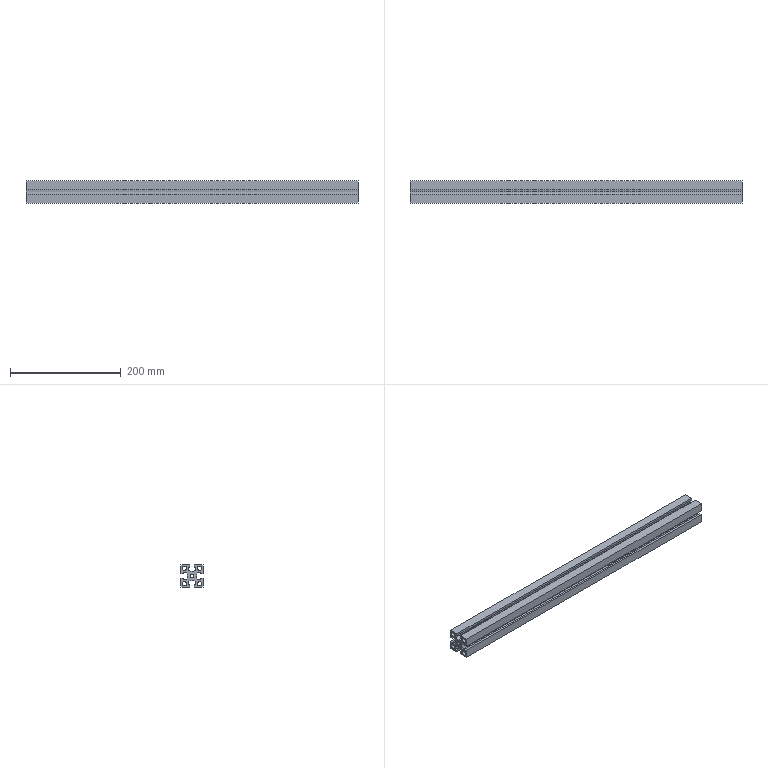Part | STEP file | PN_0069 (cross stop) | 1 solid | 49 faces | box 600 x 40 x 40 mm | volume 495706 mm3 | plane 34 | cylinder 15 | commonest cylinder face diameters 8 x8 30 x5 6.7 x2